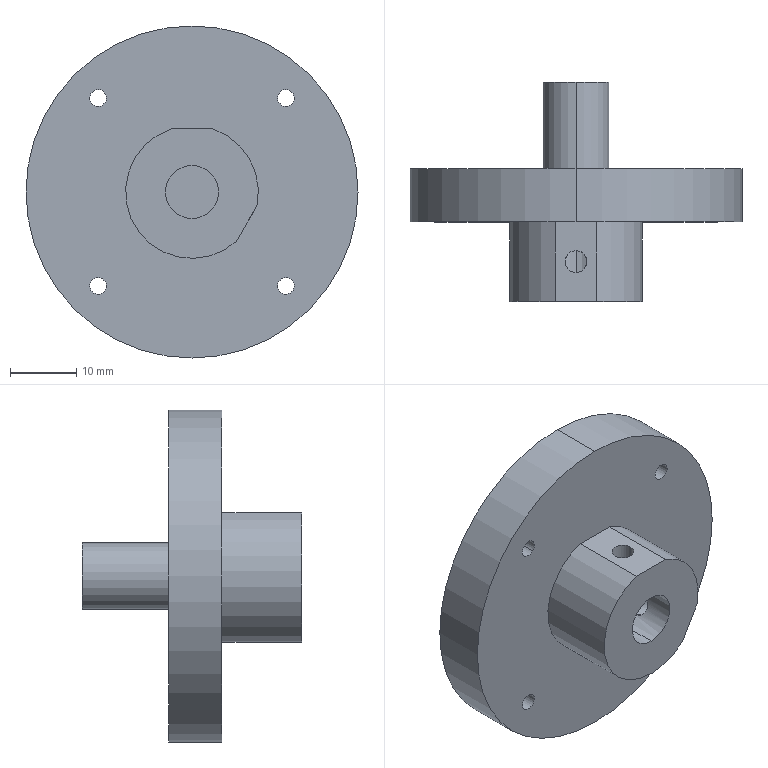Part | NX | features BREP 1 | 1 solid | 31 faces | box 50 x 33 x 50 mm | volume 19638 mm3 | cylinder 24 | plane 7 | commonest cylinder face diameters 2.5 x12 3.3 x4 8 x2 10 x2 20 x2 50 x2
STEP:
#1=CARTESIAN_POINT('',(-14.122,12.,15.412));
#2=VERTEX_POINT('',#1);
#3=CARTESIAN_POINT('',(-13.258,12.,13.258));
#4=VERTEX_POINT('',#3);
#5=CARTESIAN_POINT('',(-14.122,12.,14.162));
#6=DIRECTION('',(0.,1.,0.));
#7=DIRECTION('',(0.,0.,1.));
#8=AXIS2_PLACEMENT_3D('',#5,#6,#7);
#9=CIRCLE('',#8,1.25);
#10=EDGE_CURVE('',#2,#4,#9,.T.);
#11=ORIENTED_EDGE('',*,*,#10,.F.);
#12=CARTESIAN_POINT('',(-14.122,20.,15.412));
#13=VERTEX_POINT('',#12);
#14=CARTESIAN_POINT('',(-14.122,20.,15.412));
#15=DIRECTION('',(0.,1.,0.));
#16=VECTOR('',#15,1000.);
#17=LINE('',#14,#16);
#18=EDGE_CURVE('',#2,#13,#17,.T.);
#19=ORIENTED_EDGE('',*,*,#18,.T.);
#20=CARTESIAN_POINT('',(-13.258,20.,13.258));
#21=VERTEX_POINT('',#20);
#22=CARTESIAN_POINT('',(-14.122,20.,14.162));
#23=DIRECTION('',(0.,1.,0.));
#24=DIRECTION('',(0.,0.,1.));
#25=AXIS2_PLACEMENT_3D('',#22,#23,#24);
#26=CIRCLE('',#25,1.25);
#27=EDGE_CURVE('',#13,#21,#26,.T.);
#28=ORIENTED_EDGE('',*,*,#27,.T.);
#29=CARTESIAN_POINT('',(-13.258,10.,13.258));
#30=DIRECTION('',(0.,1.,0.));
#31=VECTOR('',#30,1000.);
#32=LINE('',#29,#31);
#33=EDGE_CURVE('',#4,#21,#32,.T.);
#34=ORIENTED_EDGE('',*,*,#33,.F.);
#35=EDGE_LOOP('',(#11,#19,#28,#34));
#36=FACE_BOUND('',#35,.T.);
#37=CARTESIAN_POINT('',(-14.122,20.,14.162));
#38=DIRECTION('',(0.,1.,0.));
#39=DIRECTION('',(0.,0.,-1.));
#40=AXIS2_PLACEMENT_3D('',#37,#38,#39);
#41=CYLINDRICAL_SURFACE('',#40,1.25);
#42=ADVANCED_FACE('',(#36),#41,.F.);
#43=CARTESIAN_POINT('',(-14.162,12.,-12.872));
#44=VERTEX_POINT('',#43);
#45=CARTESIAN_POINT('',(-13.258,12.,-13.258));
#46=VERTEX_POINT('',#45);
#47=CARTESIAN_POINT('',(-14.162,12.,-14.122));
#48=DIRECTION('',(0.,1.,0.));
#49=DIRECTION('',(0.,0.,1.));
#50=AXIS2_PLACEMENT_3D('',#47,#48,#49);
#51=CIRCLE('',#50,1.25);
#52=EDGE_CURVE('',#44,#46,#51,.T.);
#53=ORIENTED_EDGE('',*,*,#52,.F.);
#54=CARTESIAN_POINT('',(-14.162,20.,-12.872));
#55=VERTEX_POINT('',#54);
#56=CARTESIAN_POINT('',(-14.162,20.,-12.872));
#57=DIRECTION('',(0.,1.,0.));
#58=VECTOR('',#57,1000.);
#59=LINE('',#56,#58);
#60=EDGE_CURVE('',#44,#55,#59,.T.);
#61=ORIENTED_EDGE('',*,*,#60,.T.);
#62=CARTESIAN_POINT('',(-13.258,20.,-13.258));
#63=VERTEX_POINT('',#62);
#64=CARTESIAN_POINT('',(-14.162,20.,-14.122));
#65=DIRECTION('',(0.,1.,0.));
#66=DIRECTION('',(0.,0.,1.));
#67=AXIS2_PLACEMENT_3D('',#64,#65,#66);
#68=CIRCLE('',#67,1.25);
#69=EDGE_CURVE('',#55,#63,#68,.T.);
#70=ORIENTED_EDGE('',*,*,#69,.T.);
#71=CARTESIAN_POINT('',(-13.258,10.,-13.258));
#72=DIRECTION('',(0.,-1.,0.));
#73=VECTOR('',#72,1000.);
#74=LINE('',#71,#73);
#75=EDGE_CURVE('',#63,#46,#74,.T.);
#76=ORIENTED_EDGE('',*,*,#75,.T.);
#77=EDGE_LOOP('',(#53,#61,#70,#76));
#78=FACE_BOUND('',#77,.T.);
#79=CARTESIAN_POINT('',(-14.162,20.,-14.122));
#80=DIRECTION('',(0.,1.,0.));
#81=DIRECTION('',(0.,0.,-1.));
#82=AXIS2_PLACEMENT_3D('',#79,#80,#81);
#83=CYLINDRICAL_SURFACE('',#82,1.25);
#84=ADVANCED_FACE('',(#78),#83,.F.);
#85=CARTESIAN_POINT('',(14.162,12.,-12.872));
#86=VERTEX_POINT('',#85);
#87=CARTESIAN_POINT('',(15.026,12.,-15.026));
#88=VERTEX_POINT('',#87);
#89=CARTESIAN_POINT('',(14.162,12.,-14.122));
#90=DIRECTION('',(0.,1.,0.));
#91=DIRECTION('',(0.,0.,1.));
#92=AXIS2_PLACEMENT_3D('',#89,#90,#91);
#93=CIRCLE('',#92,1.25);
#94=EDGE_CURVE('',#86,#88,#93,.T.);
#95=ORIENTED_EDGE('',*,*,#94,.F.);
#96=CARTESIAN_POINT('',(14.162,20.,-12.872));
#97=VERTEX_POINT('',#96);
#98=CARTESIAN_POINT('',(14.162,20.,-12.872));
#99=DIRECTION('',(0.,1.,0.));
#100=VECTOR('',#99,1000.);
#101=LINE('',#98,#100);
#102=EDGE_CURVE('',#86,#97,#101,.T.);
#103=ORIENTED_EDGE('',*,*,#102,.T.);
#104=CARTESIAN_POINT('',(15.026,20.,-15.026));
#105=VERTEX_POINT('',#104);
#106=CARTESIAN_POINT('',(14.162,20.,-14.122));
#107=DIRECTION('',(0.,1.,0.));
#108=DIRECTION('',(0.,0.,1.));
#109=AXIS2_PLACEMENT_3D('',#106,#107,#108);
#110=CIRCLE('',#109,1.25);
#111=EDGE_CURVE('',#97,#105,#110,.T.);
#112=ORIENTED_EDGE('',*,*,#111,.T.);
#113=CARTESIAN_POINT('',(15.026,10.,-15.026));
#114=DIRECTION('',(0.,1.,0.));
#115=VECTOR('',#114,1000.);
#116=LINE('',#113,#115);
#117=EDGE_CURVE('',#88,#105,#116,.T.);
#118=ORIENTED_EDGE('',*,*,#117,.F.);
#119=EDGE_LOOP('',(#95,#103,#112,#118));
#120=FACE_BOUND('',#119,.T.);
#121=CARTESIAN_POINT('',(14.162,20.,-14.122));
#122=DIRECTION('',(0.,1.,0.));
#123=DIRECTION('',(0.,0.,-1.));
#124=AXIS2_PLACEMENT_3D('',#121,#122,#123);
#125=CYLINDRICAL_SURFACE('',#124,1.25);
#126=ADVANCED_FACE('',(#120),#125,.F.);
#127=CARTESIAN_POINT('',(14.122,12.,15.412));
#128=VERTEX_POINT('',#127);
#129=CARTESIAN_POINT('',(15.026,12.,15.026));
#130=VERTEX_POINT('',#129);
#131=CARTESIAN_POINT('',(14.122,12.,14.162));
#132=DIRECTION('',(0.,1.,0.));
#133=DIRECTION('',(0.,0.,1.));
#134=AXIS2_PLACEMENT_3D('',#131,#132,#133);
#135=CIRCLE('',#134,1.25);
#136=EDGE_CURVE('',#128,#130,#135,.T.);
#137=ORIENTED_EDGE('',*,*,#136,.F.);
#138=CARTESIAN_POINT('',(14.122,20.,15.412));
#139=VERTEX_POINT('',#138);
#140=CARTESIAN_POINT('',(14.122,20.,15.412));
#141=DIRECTION('',(0.,1.,0.));
#142=VECTOR('',#141,1000.);
#143=LINE('',#140,#142);
#144=EDGE_CURVE('',#128,#139,#143,.T.);
#145=ORIENTED_EDGE('',*,*,#144,.T.);
#146=CARTESIAN_POINT('',(15.026,20.,15.026));
#147=VERTEX_POINT('',#146);
#148=CARTESIAN_POINT('',(14.122,20.,14.162));
#149=DIRECTION('',(0.,1.,0.));
#150=DIRECTION('',(0.,0.,1.));
#151=AXIS2_PLACEMENT_3D('',#148,#149,#150);
#152=CIRCLE('',#151,1.25);
#153=EDGE_CURVE('',#139,#147,#152,.T.);
#154=ORIENTED_EDGE('',*,*,#153,.T.);
#155=CARTESIAN_POINT('',(15.026,10.,15.026));
#156=DIRECTION('',(0.,1.,0.));
#157=VECTOR('',#156,1000.);
#158=LINE('',#155,#157);
#159=EDGE_CURVE('',#130,#147,#158,.T.);
#160=ORIENTED_EDGE('',*,*,#159,.F.);
#161=EDGE_LOOP('',(#137,#145,#154,#160));
#162=FACE_BOUND('',#161,.T.);
#163=CARTESIAN_POINT('',(14.122,20.,14.162));
#164=DIRECTION('',(0.,1.,0.));
#165=DIRECTION('',(0.,0.,-1.));
#166=AXIS2_PLACEMENT_3D('',#163,#164,#165);
#167=CYLINDRICAL_SURFACE('',#166,1.25);
#168=ADVANCED_FACE('',(#162),#167,.F.);
#169=CARTESIAN_POINT('',(0.,33.,5.));
#170=VERTEX_POINT('',#169);
#171=CARTESIAN_POINT('',(0.,33.,-5.));
#172=VERTEX_POINT('',#171);
#173=CARTESIAN_POINT('',(0.,33.,0.));
#174=DIRECTION('',(0.,1.,0.));
#175=DIRECTION('',(0.,0.,1.));
#176=AXIS2_PLACEMENT_3D('',#173,#174,#175);
#177=CIRCLE('',#176,5.);
#178=EDGE_CURVE('',#170,#172,#177,.T.);
#179=ORIENTED_EDGE('',*,*,#178,.F.);
#180=CARTESIAN_POINT('',(0.,20.,5.));
#181=VERTEX_POINT('',#180);
#182=CARTESIAN_POINT('',(0.,33.,5.));
#183=DIRECTION('',(0.,-1.,0.));
#184=VECTOR('',#183,1000.);
#185=LINE('',#182,#184);
#186=EDGE_CURVE('',#181,#170,#185,.F.);
#187=ORIENTED_EDGE('',*,*,#186,.F.);
#188=CARTESIAN_POINT('',(0.,20.,-5.));
#189=VERTEX_POINT('',#188);
#190=CARTESIAN_POINT('',(0.,20.,0.));
#191=DIRECTION('',(0.,1.,0.));
#192=DIRECTION('',(0.,0.,-1.));
#193=AXIS2_PLACEMENT_3D('',#190,#191,#192);
#194=CIRCLE('',#193,5.);
#195=EDGE_CURVE('',#181,#189,#194,.T.);
#196=ORIENTED_EDGE('',*,*,#195,.T.);
#197=CARTESIAN_POINT('',(0.,33.,-5.));
#198=DIRECTION('',(0.,-1.,0.));
#199=VECTOR('',#198,1000.);
#200=LINE('',#197,#199);
#201=EDGE_CURVE('',#189,#172,#200,.F.);
#202=ORIENTED_EDGE('',*,*,#201,.T.);
#203=EDGE_LOOP('',(#179,#187,#196,#202));
#204=FACE_BOUND('',#203,.T.);
#205=CARTESIAN_POINT('',(0.,33.,0.));
#206=DIRECTION('',(0.,-1.,0.));
#207=DIRECTION('',(0.,0.,1.));
#208=AXIS2_PLACEMENT_3D('',#205,#206,#207);
#209=CYLINDRICAL_SURFACE('',#208,5.);
#210=ADVANCED_FACE('',(#204),#209,.T.);
#211=CARTESIAN_POINT('',(3.981,6.,-0.393));
#212=VERTEX_POINT('',#211);
#213=CARTESIAN_POINT('',(2.331,6.,-3.251));
#214=VERTEX_POINT('',#213);
#215=CARTESIAN_POINT('',(3.981,6.,-0.393));
#216=CARTESIAN_POINT('',(3.981,5.559,-0.393));
#217=CARTESIAN_POINT('',(3.963,4.713,-0.7955));
#218=CARTESIAN_POINT('',(3.539,4.169,-2.039));
#219=CARTESIAN_POINT('',(2.67,4.712,-3.036));
#220=CARTESIAN_POINT('',(2.331,5.559,-3.251));
#221=CARTESIAN_POINT('',(2.331,6.,-3.251));
#222=B_SPLINE_CURVE_WITH_KNOTS('',3,(#215,#216,#217,#218,#219,#220,#221),.UNSPECIFIED.,.F.,.F.,(4,1,1,1,4),(0.,0.001304,0.002607,0.003911,0.005215),.UNSPECIFIED.);
#223=EDGE_CURVE('',#212,#214,#222,.T.);
#224=ORIENTED_EDGE('',*,*,#223,.F.);
#225=CARTESIAN_POINT('',(9.052,6.,-3.321));
#226=VERTEX_POINT('',#225);
#227=CARTESIAN_POINT('',(9.485,6.,-3.571));
#228=DIRECTION('',(0.866,0.,-0.5));
#229=VECTOR('',#228,1000.);
#230=LINE('',#227,#229);
#231=EDGE_CURVE('',#226,#212,#230,.F.);
#232=ORIENTED_EDGE('',*,*,#231,.F.);
#233=CARTESIAN_POINT('',(7.402,6.,-6.179));
#234=VERTEX_POINT('',#233);
#235=CARTESIAN_POINT('',(8.227,6.,-4.75));
#236=DIRECTION('',(0.866,0.,-0.5));
#237=DIRECTION('',(0.5,0.,0.866));
#238=AXIS2_PLACEMENT_3D('',#235,#236,#237);
#239=CIRCLE('',#238,1.65);
#240=EDGE_CURVE('',#226,#234,#239,.T.);
#241=ORIENTED_EDGE('',*,*,#240,.T.);
#242=CARTESIAN_POINT('',(7.835,6.,-6.429));
#243=DIRECTION('',(0.866,0.,-0.5));
#244=VECTOR('',#243,1000.);
#245=LINE('',#242,#244);
#246=EDGE_CURVE('',#234,#214,#245,.F.);
#247=ORIENTED_EDGE('',*,*,#246,.T.);
#248=EDGE_LOOP('',(#224,#232,#241,#247));
#249=FACE_BOUND('',#248,.T.);
#250=CARTESIAN_POINT('',(8.66,6.,-5.));
#251=DIRECTION('',(0.866,0.,-0.5));
#252=DIRECTION('',(0.5,0.,0.866));
#253=AXIS2_PLACEMENT_3D('',#250,#251,#252);
#254=CYLINDRICAL_SURFACE('',#253,1.65);
#255=ADVANCED_FACE('',(#249),#254,.F.);
#256=CARTESIAN_POINT('',(-1.65,6.,3.644));
#257=VERTEX_POINT('',#256);
#258=CARTESIAN_POINT('',(0.,4.35,4.));
#259=VERTEX_POINT('',#258);
#260=CARTESIAN_POINT('',(-1.65,6.,3.644));
#261=CARTESIAN_POINT('',(-1.65,5.118,3.644));
#262=CARTESIAN_POINT('',(-0.8824,4.35,4.));
#263=CARTESIAN_POINT('',(0.,4.35,4.));
#264=B_SPLINE_CURVE_WITH_KNOTS('',3,(#260,#261,#262,#263),.UNSPECIFIED.,.F.,.F.,(4,4),(0.,0.002607),.UNSPECIFIED.);
#265=EDGE_CURVE('',#257,#259,#264,.T.);
#266=ORIENTED_EDGE('',*,*,#265,.F.);
#267=CARTESIAN_POINT('',(-1.65,6.,9.5));
#268=VERTEX_POINT('',#267);
#269=CARTESIAN_POINT('',(-1.65,6.,10.));
#270=DIRECTION('',(0.,0.,1.));
#271=VECTOR('',#270,1000.);
#272=LINE('',#269,#271);
#273=EDGE_CURVE('',#257,#268,#272,.T.);
#274=ORIENTED_EDGE('',*,*,#273,.T.);
#275=CARTESIAN_POINT('',(1.65,6.,9.5));
#276=VERTEX_POINT('',#275);
#277=CARTESIAN_POINT('',(0.,6.,9.5));
#278=DIRECTION('',(0.,0.,1.));
#279=DIRECTION('',(-1.,0.,0.));
#280=AXIS2_PLACEMENT_3D('',#277,#278,#279);
#281=CIRCLE('',#280,1.65);
#282=EDGE_CURVE('',#268,#276,#281,.T.);
#283=ORIENTED_EDGE('',*,*,#282,.T.);
#284=CARTESIAN_POINT('',(1.65,6.,3.644));
#285=VERTEX_POINT('',#284);
#286=CARTESIAN_POINT('',(1.65,6.,10.));
#287=DIRECTION('',(0.,0.,1.));
#288=VECTOR('',#287,1000.);
#289=LINE('',#286,#288);
#290=EDGE_CURVE('',#285,#276,#289,.T.);
#291=ORIENTED_EDGE('',*,*,#290,.F.);
#292=CARTESIAN_POINT('',(0.,4.35,4.));
#293=CARTESIAN_POINT('',(0.8823,4.35,4.));
#294=CARTESIAN_POINT('',(1.65,5.118,3.644));
#295=CARTESIAN_POINT('',(1.65,6.,3.644));
#296=B_SPLINE_CURVE_WITH_KNOTS('',3,(#292,#293,#294,#295),.UNSPECIFIED.,.F.,.F.,(4,4),(0.,0.002607),.UNSPECIFIED.);
#297=EDGE_CURVE('',#259,#285,#296,.T.);
#298=ORIENTED_EDGE('',*,*,#297,.F.);
#299=EDGE_LOOP('',(#266,#274,#283,#291,#298));
#300=FACE_BOUND('',#299,.T.);
#301=CARTESIAN_POINT('',(0.,6.,10.));
#302=DIRECTION('',(0.,0.,1.));
#303=DIRECTION('',(-1.,0.,0.));
#304=AXIS2_PLACEMENT_3D('',#301,#302,#303);
#305=CYLINDRICAL_SURFACE('',#304,1.65);
#306=ADVANCED_FACE('',(#300),#305,.F.);
#307=CARTESIAN_POINT('',(0.,11.,4.));
#308=VERTEX_POINT('',#307);
#309=CARTESIAN_POINT('',(0.,11.,-4.));
#310=VERTEX_POINT('',#309);
#311=CARTESIAN_POINT('',(0.,11.,0.));
#312=DIRECTION('',(0.,-1.,0.));
#313=DIRECTION('',(0.,0.,-1.));
#314=AXIS2_PLACEMENT_3D('',#311,#312,#313);
#315=CIRCLE('',#314,4.);
#316=EDGE_CURVE('',#308,#310,#315,.T.);
#317=ORIENTED_EDGE('',*,*,#316,.F.);
#318=CARTESIAN_POINT('',(0.,7.65,4.));
#319=VERTEX_POINT('',#318);
#320=CARTESIAN_POINT('',(0.,11.,4.));
#321=DIRECTION('',(0.,-1.,0.));
#322=VECTOR('',#321,1000.);
#323=LINE('',#320,#322);
#324=EDGE_CURVE('',#319,#308,#323,.F.);
#325=ORIENTED_EDGE('',*,*,#324,.F.);
#326=CARTESIAN_POINT('',(0.,7.65,4.));
#327=CARTESIAN_POINT('',(-0.8823,7.65,4.));
#328=CARTESIAN_POINT('',(-1.65,6.882,3.644));
#329=CARTESIAN_POINT('',(-1.65,6.,3.644));
#330=B_SPLINE_CURVE_WITH_KNOTS('',3,(#326,#327,#328,#329),.UNSPECIFIED.,.F.,.F.,(4,4),(0.,0.002607),.UNSPECIFIED.);
#331=EDGE_CURVE('',#319,#257,#330,.T.);
#332=ORIENTED_EDGE('',*,*,#331,.T.);
#333=ORIENTED_EDGE('',*,*,#265,.T.);
#334=CARTESIAN_POINT('',(0.,0.,4.));
#335=VERTEX_POINT('',#334);
#336=CARTESIAN_POINT('',(0.,11.,4.));
#337=DIRECTION('',(0.,-1.,0.));
#338=VECTOR('',#337,1000.);
#339=LINE('',#336,#338);
#340=EDGE_CURVE('',#259,#335,#339,.T.);
#341=ORIENTED_EDGE('',*,*,#340,.T.);
#342=CARTESIAN_POINT('',(0.,0.,-4.));
#343=VERTEX_POINT('',#342);
#344=CARTESIAN_POINT('',(0.,0.,0.));
#345=DIRECTION('',(0.,-1.,0.));
#346=DIRECTION('',(0.,0.,-1.));
#347=AXIS2_PLACEMENT_3D('',#344,#345,#346);
#348=CIRCLE('',#347,4.);
#349=EDGE_CURVE('',#335,#343,#348,.T.);
#350=ORIENTED_EDGE('',*,*,#349,.T.);
#351=CARTESIAN_POINT('',(0.,11.,-4.));
#352=DIRECTION('',(0.,-1.,0.));
#353=VECTOR('',#352,1000.);
#354=LINE('',#351,#353);
#355=EDGE_CURVE('',#343,#310,#354,.F.);
#356=ORIENTED_EDGE('',*,*,#355,.T.);
#357=EDGE_LOOP('',(#317,#325,#332,#333,#341,#350,#356));
#358=FACE_BOUND('',#357,.T.);
#359=CARTESIAN_POINT('',(0.,11.,0.));
#360=DIRECTION('',(0.,-1.,0.));
#361=DIRECTION('',(0.,0.,1.));
#362=AXIS2_PLACEMENT_3D('',#359,#360,#361);
#363=CYLINDRICAL_SURFACE('',#362,4.);
#364=ADVANCED_FACE('',(#358),#363,.F.);
#365=CARTESIAN_POINT('',(0.,12.,25.));
#366=VERTEX_POINT('',#365);
#367=CARTESIAN_POINT('',(0.,12.,-25.));
#368=VERTEX_POINT('',#367);
#369=CARTESIAN_POINT('',(0.,12.,0.));
#370=DIRECTION('',(0.,1.,0.));
#371=DIRECTION('',(0.,0.,1.));
#372=AXIS2_PLACEMENT_3D('',#369,#370,#371);
#373=CIRCLE('',#372,25.);
#374=EDGE_CURVE('',#366,#368,#373,.T.);
#375=ORIENTED_EDGE('',*,*,#374,.T.);
#376=CARTESIAN_POINT('',(0.,20.,-25.));
#377=VERTEX_POINT('',#376);
#378=CARTESIAN_POINT('',(0.,81.449,-25.));
#379=DIRECTION('',(0.,1.,0.));
#380=VECTOR('',#379,1000.);
#381=LINE('',#378,#380);
#382=EDGE_CURVE('',#368,#377,#381,.T.);
#383=ORIENTED_EDGE('',*,*,#382,.T.);
#384=CARTESIAN_POINT('',(0.,20.,25.));
#385=VERTEX_POINT('',#384);
#386=CARTESIAN_POINT('',(0.,20.,0.));
#387=DIRECTION('',(0.,1.,0.));
#388=DIRECTION('',(0.,0.,1.));
#389=AXIS2_PLACEMENT_3D('',#386,#387,#388);
#390=CIRCLE('',#389,25.);
#391=EDGE_CURVE('',#385,#377,#390,.T.);
#392=ORIENTED_EDGE('',*,*,#391,.F.);
#393=CARTESIAN_POINT('',(0.,81.449,25.));
#394=DIRECTION('',(0.,1.,0.));
#395=VECTOR('',#394,1000.);
#396=LINE('',#393,#395);
#397=EDGE_CURVE('',#366,#385,#396,.T.);
#398=ORIENTED_EDGE('',*,*,#397,.F.);
#399=EDGE_LOOP('',(#375,#383,#392,#398));
#400=FACE_BOUND('',#399,.T.);
#401=CARTESIAN_POINT('',(0.,81.449,0.));
#402=DIRECTION('',(0.,1.,0.));
#403=DIRECTION('',(0.,0.,-1.));
#404=AXIS2_PLACEMENT_3D('',#401,#402,#403);
#405=CYLINDRICAL_SURFACE('',#404,25.);
#406=ADVANCED_FACE('',(#400),#405,.T.);
#407=CARTESIAN_POINT('',(-15.026,20.,-15.026));
#408=VERTEX_POINT('',#407);
#409=CARTESIAN_POINT('',(-14.122,20.,-14.162));
#410=DIRECTION('',(0.,1.,0.));
#411=DIRECTION('',(0.,0.,1.));
#412=AXIS2_PLACEMENT_3D('',#409,#410,#411);
#413=CIRCLE('',#412,1.25);
#414=EDGE_CURVE('',#63,#408,#413,.T.);
#415=ORIENTED_EDGE('',*,*,#414,.F.);
#416=ORIENTED_EDGE('',*,*,#69,.F.);
#417=CARTESIAN_POINT('',(-14.162,20.,-14.122));
#418=DIRECTION('',(0.,1.,0.));
#419=DIRECTION('',(0.,0.,1.));
#420=AXIS2_PLACEMENT_3D('',#417,#418,#419);
#421=CIRCLE('',#420,1.25);
#422=EDGE_CURVE('',#408,#55,#421,.T.);
#423=ORIENTED_EDGE('',*,*,#422,.F.);
#424=EDGE_LOOP('',(#415,#416,#423));
#425=FACE_BOUND('',#424,.T.);
#426=CARTESIAN_POINT('',(13.258,20.,-13.258));
#427=VERTEX_POINT('',#426);
#428=CARTESIAN_POINT('',(14.122,20.,-14.162));
#429=DIRECTION('',(0.,1.,0.));
#430=DIRECTION('',(0.,0.,1.));
#431=AXIS2_PLACEMENT_3D('',#428,#429,#430);
#432=CIRCLE('',#431,1.25);
#433=EDGE_CURVE('',#105,#427,#432,.T.);
#434=ORIENTED_EDGE('',*,*,#433,.F.);
#435=ORIENTED_EDGE('',*,*,#111,.F.);
#436=CARTESIAN_POINT('',(14.162,20.,-14.122));
#437=DIRECTION('',(0.,1.,0.));
#438=DIRECTION('',(0.,0.,1.));
#439=AXIS2_PLACEMENT_3D('',#436,#437,#438);
#440=CIRCLE('',#439,1.25);
#441=EDGE_CURVE('',#427,#97,#440,.T.);
#442=ORIENTED_EDGE('',*,*,#441,.F.);
#443=EDGE_LOOP('',(#434,#435,#442));
#444=FACE_BOUND('',#443,.T.);
#445=CARTESIAN_POINT('',(13.258,20.,13.258));
#446=VERTEX_POINT('',#445);
#447=CARTESIAN_POINT('',(14.162,20.,14.122));
#448=DIRECTION('',(0.,1.,0.));
#449=DIRECTION('',(0.,0.,1.));
#450=AXIS2_PLACEMENT_3D('',#447,#448,#449);
#451=CIRCLE('',#450,1.25);
#452=EDGE_CURVE('',#147,#446,#451,.T.);
#453=ORIENTED_EDGE('',*,*,#452,.F.);
#454=ORIENTED_EDGE('',*,*,#153,.F.);
#455=CARTESIAN_POINT('',(14.122,20.,14.162));
#456=DIRECTION('',(0.,1.,0.));
#457=DIRECTION('',(0.,0.,1.));
#458=AXIS2_PLACEMENT_3D('',#455,#456,#457);
#459=CIRCLE('',#458,1.25);
#460=EDGE_CURVE('',#446,#139,#459,.T.);
#461=ORIENTED_EDGE('',*,*,#460,.F.);
#462=EDGE_LOOP('',(#453,#454,#461));
#463=FACE_BOUND('',#462,.T.);
#464=CARTESIAN_POINT('',(0.,20.,0.));
#465=DIRECTION('',(0.,1.,0.));
#466=DIRECTION('',(0.,0.,-1.));
#467=AXIS2_PLACEMENT_3D('',#464,#465,#466);
#468=CIRCLE('',#467,5.);
#469=EDGE_CURVE('',#189,#181,#468,.T.);
#470=ORIENTED_EDGE('',*,*,#469,.F.);
#471=ORIENTED_EDGE('',*,*,#195,.F.);
#472=EDGE_LOOP('',(#470,#471));
#473=FACE_BOUND('',#472,.T.);
#474=ORIENTED_EDGE('',*,*,#391,.T.);
#475=CARTESIAN_POINT('',(0.,20.,0.));
#476=DIRECTION('',(0.,1.,0.));
#477=DIRECTION('',(0.,0.,1.));
#478=AXIS2_PLACEMENT_3D('',#475,#476,#477);
#479=CIRCLE('',#478,25.);
#480=EDGE_CURVE('',#377,#385,#479,.T.);
#481=ORIENTED_EDGE('',*,*,#480,.T.);
#482=EDGE_LOOP('',(#474,#481));
#483=FACE_BOUND('',#482,.T.);
#484=CARTESIAN_POINT('',(-15.026,20.,15.026));
#485=VERTEX_POINT('',#484);
#486=CARTESIAN_POINT('',(-14.122,20.,14.162));
#487=DIRECTION('',(0.,1.,0.));
#488=DIRECTION('',(0.,0.,1.));
#489=AXIS2_PLACEMENT_3D('',#486,#487,#488);
#490=CIRCLE('',#489,1.25);
#491=EDGE_CURVE('',#485,#13,#490,.T.);
#492=ORIENTED_EDGE('',*,*,#491,.F.);
#493=CARTESIAN_POINT('',(-14.162,20.,14.122));
#494=DIRECTION('',(0.,1.,0.));
#495=DIRECTION('',(0.,0.,1.));
#496=AXIS2_PLACEMENT_3D('',#493,#494,#495);
#497=CIRCLE('',#496,1.25);
#498=EDGE_CURVE('',#21,#485,#497,.T.);
#499=ORIENTED_EDGE('',*,*,#498,.F.);
#500=ORIENTED_EDGE('',*,*,#27,.F.);
#501=EDGE_LOOP('',(#492,#499,#500));
#502=FACE_BOUND('',#501,.T.);
#503=CARTESIAN_POINT('',(0.,20.,0.));
#504=DIRECTION('',(0.,-1.,0.));
#505=DIRECTION('',(0.,0.,1.));
#506=AXIS2_PLACEMENT_3D('',#503,#504,#505);
#507=PLANE('',#506);
#508=ADVANCED_FACE('',(#425,#444,#463,#473,#483,#502),#507,.F.);
#509=CARTESIAN_POINT('',(3.122,0.,9.5));
#510=VERTEX_POINT('',#509);
#511=CARTESIAN_POINT('',(9.788,0.,-2.046));
#512=VERTEX_POINT('',#511);
#513=CARTESIAN_POINT('',(0.,0.,0.));
#514=DIRECTION('',(0.,1.,0.));
#515=DIRECTION('',(0.,0.,1.));
#516=AXIS2_PLACEMENT_3D('',#513,#514,#515);
#517=CIRCLE('',#516,10.);
#518=EDGE_CURVE('',#510,#512,#517,.T.);
#519=ORIENTED_EDGE('',*,*,#518,.T.);
#520=CARTESIAN_POINT('',(9.788,12.,-2.046));
#521=VERTEX_POINT('',#520);
#522=CARTESIAN_POINT('',(9.788,18.245,-2.046));
#523=DIRECTION('',(0.,-1.,0.));
#524=VECTOR('',#523,1000.);
#525=LINE('',#522,#524);
#526=EDGE_CURVE('',#521,#512,#525,.T.);
#527=ORIENTED_EDGE('',*,*,#526,.F.);
#528=CARTESIAN_POINT('',(3.122,12.,9.5));
#529=VERTEX_POINT('',#528);
#530=CARTESIAN_POINT('',(0.,12.,0.));
#531=DIRECTION('',(0.,1.,0.));
#532=DIRECTION('',(0.,0.,1.));
#533=AXIS2_PLACEMENT_3D('',#530,#531,#532);
#534=CIRCLE('',#533,10.);
#535=EDGE_CURVE('',#529,#521,#534,.T.);
#536=ORIENTED_EDGE('',*,*,#535,.F.);
#537=CARTESIAN_POINT('',(3.122,18.265,9.5));
#538=DIRECTION('',(0.,-1.,0.));
#539=VECTOR('',#538,1000.);
#540=LINE('',#537,#539);
#541=EDGE_CURVE('',#529,#510,#540,.T.);
#542=ORIENTED_EDGE('',*,*,#541,.T.);
#543=EDGE_LOOP('',(#519,#527,#536,#542));
#544=FACE_BOUND('',#543,.T.);
#545=CARTESIAN_POINT('',(0.,81.449,0.));
#546=DIRECTION('',(0.,1.,0.));
#547=DIRECTION('',(0.,0.,-1.));
#548=AXIS2_PLACEMENT_3D('',#545,#546,#547);
#549=CYLINDRICAL_SURFACE('',#548,10.);
#550=ADVANCED_FACE('',(#544),#549,.T.);
#551=ORIENTED_EDGE('',*,*,#382,.F.);
#552=CARTESIAN_POINT('',(0.,12.,0.));
#553=DIRECTION('',(0.,1.,0.));
#554=DIRECTION('',(0.,0.,1.));
#555=AXIS2_PLACEMENT_3D('',#552,#553,#554);
#556=CIRCLE('',#555,25.);
#557=EDGE_CURVE('',#368,#366,#556,.T.);
#558=ORIENTED_EDGE('',*,*,#557,.T.);
#559=ORIENTED_EDGE('',*,*,#397,.T.);
#560=ORIENTED_EDGE('',*,*,#480,.F.);
#561=EDGE_LOOP('',(#551,#558,#559,#560));
#562=FACE_BOUND('',#561,.T.);
#563=CARTESIAN_POINT('',(0.,81.449,0.));
#564=DIRECTION('',(0.,1.,0.));
#565=DIRECTION('',(0.,0.,-1.));
#566=AXIS2_PLACEMENT_3D('',#563,#564,#565);
#567=CYLINDRICAL_SURFACE('',#566,25.);
#568=ADVANCED_FACE('',(#562),#567,.T.);
#569=CARTESIAN_POINT('',(-15.026,12.,-15.026));
#570=VERTEX_POINT('',#569);
#571=CARTESIAN_POINT('',(-14.162,12.,-14.122));
#572=DIRECTION('',(0.,1.,0.));
#573=DIRECTION('',(0.,0.,1.));
#574=AXIS2_PLACEMENT_3D('',#571,#572,#573);
#575=CIRCLE('',#574,1.25);
#576=EDGE_CURVE('',#570,#44,#575,.T.);
#577=ORIENTED_EDGE('',*,*,#576,.T.);
#578=ORIENTED_EDGE('',*,*,#52,.T.);
#579=CARTESIAN_POINT('',(-14.122,12.,-14.162));
#580=DIRECTION('',(0.,1.,0.));
#581=DIRECTION('',(0.,0.,1.));
#582=AXIS2_PLACEMENT_3D('',#579,#580,#581);
#583=CIRCLE('',#582,1.25);
#584=EDGE_CURVE('',#46,#570,#583,.T.);
#585=ORIENTED_EDGE('',*,*,#584,.T.);
#586=EDGE_LOOP('',(#577,#578,#585));
#587=FACE_BOUND('',#586,.T.);
#588=CARTESIAN_POINT('',(13.258,12.,-13.258));
#589=VERTEX_POINT('',#588);
#590=CARTESIAN_POINT('',(14.122,12.,-14.162));
#591=DIRECTION('',(0.,1.,0.));
#592=DIRECTION('',(0.,0.,1.));
#593=AXIS2_PLACEMENT_3D('',#590,#591,#592);
#594=CIRCLE('',#593,1.25);
#595=EDGE_CURVE('',#88,#589,#594,.T.);
#596=ORIENTED_EDGE('',*,*,#595,.T.);
#597=CARTESIAN_POINT('',(14.162,12.,-14.122));
#598=DIRECTION('',(0.,1.,0.));
#599=DIRECTION('',(0.,0.,1.));
#600=AXIS2_PLACEMENT_3D('',#597,#598,#599);
#601=CIRCLE('',#600,1.25);
#602=EDGE_CURVE('',#589,#86,#601,.T.);
#603=ORIENTED_EDGE('',*,*,#602,.T.);
#604=ORIENTED_EDGE('',*,*,#94,.T.);
#605=EDGE_LOOP('',(#596,#603,#604));
#606=FACE_BOUND('',#605,.T.);
#607=CARTESIAN_POINT('',(13.258,12.,13.258));
#608=VERTEX_POINT('',#607);
#609=CARTESIAN_POINT('',(14.162,12.,14.122));
#610=DIRECTION('',(0.,1.,0.));
#611=DIRECTION('',(0.,0.,1.));
#612=AXIS2_PLACEMENT_3D('',#609,#610,#611);
#613=CIRCLE('',#612,1.25);
#614=EDGE_CURVE('',#130,#608,#613,.T.);
#615=ORIENTED_EDGE('',*,*,#614,.T.);
#616=CARTESIAN_POINT('',(14.122,12.,14.162));
#617=DIRECTION('',(0.,1.,0.));
#618=DIRECTION('',(0.,0.,1.));
#619=AXIS2_PLACEMENT_3D('',#616,#617,#618);
#620=CIRCLE('',#619,1.25);
#621=EDGE_CURVE('',#608,#128,#620,.T.);
#622=ORIENTED_EDGE('',*,*,#621,.T.);
#623=ORIENTED_EDGE('',*,*,#136,.T.);
#624=EDGE_LOOP('',(#615,#622,#623));
#625=FACE_BOUND('',#624,.T.);
#626=CARTESIAN_POINT('',(-15.026,12.,15.026));
#627=VERTEX_POINT('',#626);
#628=CARTESIAN_POINT('',(-14.162,12.,14.122));
#629=DIRECTION('',(0.,1.,0.));
#630=DIRECTION('',(0.,0.,1.));
#631=AXIS2_PLACEMENT_3D('',#628,#629,#630);
#632=CIRCLE('',#631,1.25);
#633=EDGE_CURVE('',#4,#627,#632,.T.);
#634=ORIENTED_EDGE('',*,*,#633,.T.);
#635=CARTESIAN_POINT('',(-14.122,12.,14.162));
#636=DIRECTION('',(0.,1.,0.));
#637=DIRECTION('',(0.,0.,1.));
#638=AXIS2_PLACEMENT_3D('',#635,#636,#637);
#639=CIRCLE('',#638,1.25);
#640=EDGE_CURVE('',#627,#2,#639,.T.);
#641=ORIENTED_EDGE('',*,*,#640,.T.);
#642=ORIENTED_EDGE('',*,*,#10,.T.);
#643=EDGE_LOOP('',(#634,#641,#642));
#644=FACE_BOUND('',#643,.T.);
#645=ORIENTED_EDGE('',*,*,#374,.F.);
#646=ORIENTED_EDGE('',*,*,#557,.F.);
#647=EDGE_LOOP('',(#645,#646));
#648=FACE_BOUND('',#647,.T.);
#649=ORIENTED_EDGE('',*,*,#535,.T.);
#650=CARTESIAN_POINT('',(6.666,12.,-7.454));
#651=VERTEX_POINT('',#650);
#652=CARTESIAN_POINT('',(9.788,12.,-2.046));
#653=DIRECTION('',(-0.5,0.,-0.866));
#654=VECTOR('',#653,1000.);
#655=LINE('',#652,#654);
#656=EDGE_CURVE('',#521,#651,#655,.T.);
#657=ORIENTED_EDGE('',*,*,#656,.T.);
#658=CARTESIAN_POINT('',(-3.122,12.,9.5));
#659=VERTEX_POINT('',#658);
#660=CARTESIAN_POINT('',(0.,12.,0.));
#661=DIRECTION('',(0.,1.,0.));
#662=DIRECTION('',(0.,0.,1.));
#663=AXIS2_PLACEMENT_3D('',#660,#661,#662);
#664=CIRCLE('',#663,10.);
#665=EDGE_CURVE('',#651,#659,#664,.T.);
#666=ORIENTED_EDGE('',*,*,#665,.T.);
#667=CARTESIAN_POINT('',(-3.122,12.,9.5));
#668=DIRECTION('',(1.,0.,0.));
#669=VECTOR('',#668,1000.);
#670=LINE('',#667,#669);
#671=EDGE_CURVE('',#659,#529,#670,.T.);
#672=ORIENTED_EDGE('',*,*,#671,.T.);
#673=EDGE_LOOP('',(#649,#657,#666,#672));
#674=FACE_BOUND('',#673,.T.);
#675=CARTESIAN_POINT('',(25.,12.,0.));
#676=DIRECTION('',(0.,1.,0.));
#677=DIRECTION('',(0.,0.,-1.));
#678=AXIS2_PLACEMENT_3D('',#675,#676,#677);
#679=PLANE('',#678);
#680=ADVANCED_FACE('',(#587,#606,#625,#644,#648,#674),#679,.F.);
#681=ORIENTED_EDGE('',*,*,#665,.F.);
#682=CARTESIAN_POINT('',(6.666,0.,-7.454));
#683=VERTEX_POINT('',#682);
#684=CARTESIAN_POINT('',(6.666,18.245,-7.454));
#685=DIRECTION('',(0.,-1.,0.));
#686=VECTOR('',#685,1000.);
#687=LINE('',#684,#686);
#688=EDGE_CURVE('',#651,#683,#687,.T.);
#689=ORIENTED_EDGE('',*,*,#688,.T.);
#690=CARTESIAN_POINT('',(-3.122,0.,9.5));
#691=VERTEX_POINT('',#690);
#692=CARTESIAN_POINT('',(0.,0.,0.));
#693=DIRECTION('',(0.,1.,0.));
#694=DIRECTION('',(0.,0.,1.));
#695=AXIS2_PLACEMENT_3D('',#692,#693,#694);
#696=CIRCLE('',#695,10.);
#697=EDGE_CURVE('',#683,#691,#696,.T.);
#698=ORIENTED_EDGE('',*,*,#697,.T.);
#699=CARTESIAN_POINT('',(-3.122,18.265,9.5));
#700=DIRECTION('',(0.,-1.,0.));
#701=VECTOR('',#700,1000.);
#702=LINE('',#699,#701);
#703=EDGE_CURVE('',#659,#691,#702,.T.);
#704=ORIENTED_EDGE('',*,*,#703,.F.);
#705=EDGE_LOOP('',(#681,#689,#698,#704));
#706=FACE_BOUND('',#705,.T.);
#707=CARTESIAN_POINT('',(0.,81.449,0.));
#708=DIRECTION('',(0.,1.,0.));
#709=DIRECTION('',(0.,0.,-1.));
#710=AXIS2_PLACEMENT_3D('',#707,#708,#709);
#711=CYLINDRICAL_SURFACE('',#710,10.);
#712=ADVANCED_FACE('',(#706),#711,.T.);
#713=CARTESIAN_POINT('',(0.,0.,0.));
#714=DIRECTION('',(0.,-1.,0.));
#715=DIRECTION('',(0.,0.,-1.));
#716=AXIS2_PLACEMENT_3D('',#713,#714,#715);
#717=CIRCLE('',#716,4.);
#718=EDGE_CURVE('',#343,#335,#717,.T.);
#719=ORIENTED_EDGE('',*,*,#718,.F.);
#720=ORIENTED_EDGE('',*,*,#349,.F.);
#721=EDGE_LOOP('',(#719,#720));
#722=FACE_BOUND('',#721,.T.);
#723=ORIENTED_EDGE('',*,*,#697,.F.);
#724=CARTESIAN_POINT('',(9.788,0.,-2.046));
#725=DIRECTION('',(-0.5,0.,-0.866));
#726=VECTOR('',#725,1000.);
#727=LINE('',#724,#726);
#728=EDGE_CURVE('',#512,#683,#727,.T.);
#729=ORIENTED_EDGE('',*,*,#728,.F.);
#730=ORIENTED_EDGE('',*,*,#518,.F.);
#731=CARTESIAN_POINT('',(-3.122,0.,9.5));
#732=DIRECTION('',(1.,0.,0.));
#733=VECTOR('',#732,1000.);
#734=LINE('',#731,#733);
#735=EDGE_CURVE('',#691,#510,#734,.T.);
#736=ORIENTED_EDGE('',*,*,#735,.F.);
#737=EDGE_LOOP('',(#723,#729,#730,#736));
#738=FACE_BOUND('',#737,.T.);
#739=CARTESIAN_POINT('',(10.,0.,0.));
#740=DIRECTION('',(0.,1.,0.));
#741=DIRECTION('',(0.,0.,-1.));
#742=AXIS2_PLACEMENT_3D('',#739,#740,#741);
#743=PLANE('',#742);
#744=ADVANCED_FACE('',(#722,#738),#743,.F.);
#745=ORIENTED_EDGE('',*,*,#324,.T.);
#746=CARTESIAN_POINT('',(0.,11.,0.));
#747=DIRECTION('',(0.,-1.,0.));
#748=DIRECTION('',(0.,0.,-1.));
#749=AXIS2_PLACEMENT_3D('',#746,#747,#748);
#750=CIRCLE('',#749,4.);
#751=EDGE_CURVE('',#310,#308,#750,.T.);
#752=ORIENTED_EDGE('',*,*,#751,.F.);
#753=ORIENTED_EDGE('',*,*,#355,.F.);
#754=ORIENTED_EDGE('',*,*,#718,.T.);
#755=ORIENTED_EDGE('',*,*,#340,.F.);
#756=ORIENTED_EDGE('',*,*,#297,.T.);
#757=CARTESIAN_POINT('',(1.65,6.,3.644));
#758=CARTESIAN_POINT('',(1.65,6.882,3.644));
#759=CARTESIAN_POINT('',(0.8824,7.65,4.));
#760=CARTESIAN_POINT('',(0.,7.65,4.));
#761=B_SPLINE_CURVE_WITH_KNOTS('',3,(#757,#758,#759,#760),.UNSPECIFIED.,.F.,.F.,(4,4),(0.,0.002607),.UNSPECIFIED.);
#762=EDGE_CURVE('',#285,#319,#761,.T.);
#763=ORIENTED_EDGE('',*,*,#762,.T.);
#764=EDGE_LOOP('',(#745,#752,#753,#754,#755,#756,#763));
#765=FACE_BOUND('',#764,.T.);
#766=CARTESIAN_POINT('',(2.331,6.,-3.251));
#767=CARTESIAN_POINT('',(2.331,6.441,-3.251));
#768=CARTESIAN_POINT('',(2.671,7.287,-3.034));
#769=CARTESIAN_POINT('',(3.536,7.831,-2.045));
#770=CARTESIAN_POINT('',(3.964,7.288,-0.7946));
#771=CARTESIAN_POINT('',(3.981,6.441,-0.393));
#772=CARTESIAN_POINT('',(3.981,6.,-0.393));
#773=B_SPLINE_CURVE_WITH_KNOTS('',3,(#766,#767,#768,#769,#770,#771,#772),.UNSPECIFIED.,.F.,.F.,(4,1,1,1,4),(0.,0.001304,0.002607,0.003911,0.005215),.UNSPECIFIED.);
#774=EDGE_CURVE('',#214,#212,#773,.T.);
#775=ORIENTED_EDGE('',*,*,#774,.T.);
#776=ORIENTED_EDGE('',*,*,#223,.T.);
#777=EDGE_LOOP('',(#775,#776));
#778=FACE_BOUND('',#777,.T.);
#779=CARTESIAN_POINT('',(0.,11.,0.));
#780=DIRECTION('',(0.,-1.,0.));
#781=DIRECTION('',(0.,0.,1.));
#782=AXIS2_PLACEMENT_3D('',#779,#780,#781);
#783=CYLINDRICAL_SURFACE('',#782,4.);
#784=ADVANCED_FACE('',(#765,#778),#783,.F.);
#785=ORIENTED_EDGE('',*,*,#751,.T.);
#786=ORIENTED_EDGE('',*,*,#316,.T.);
#787=EDGE_LOOP('',(#785,#786));
#788=FACE_BOUND('',#787,.T.);
#789=CARTESIAN_POINT('',(0.,11.,0.));
#790=DIRECTION('',(0.,-1.,0.));
#791=DIRECTION('',(0.,0.,1.));
#792=AXIS2_PLACEMENT_3D('',#789,#790,#791);
#793=PLANE('',#792);
#794=ADVANCED_FACE('',(#788),#793,.T.);
#795=ORIENTED_EDGE('',*,*,#273,.F.);
#796=ORIENTED_EDGE('',*,*,#331,.F.);
#797=ORIENTED_EDGE('',*,*,#762,.F.);
#798=ORIENTED_EDGE('',*,*,#290,.T.);
#799=CARTESIAN_POINT('',(0.,6.,9.5));
#800=DIRECTION('',(0.,0.,1.));
#801=DIRECTION('',(-1.,0.,0.));
#802=AXIS2_PLACEMENT_3D('',#799,#800,#801);
#803=CIRCLE('',#802,1.65);
#804=EDGE_CURVE('',#276,#268,#803,.T.);
#805=ORIENTED_EDGE('',*,*,#804,.T.);
#806=EDGE_LOOP('',(#795,#796,#797,#798,#805));
#807=FACE_BOUND('',#806,.T.);
#808=CARTESIAN_POINT('',(0.,6.,10.));
#809=DIRECTION('',(0.,0.,1.));
#810=DIRECTION('',(-1.,0.,0.));
#811=AXIS2_PLACEMENT_3D('',#808,#809,#810);
#812=CYLINDRICAL_SURFACE('',#811,1.65);
#813=ADVANCED_FACE('',(#807),#812,.F.);
#814=ORIENTED_EDGE('',*,*,#703,.T.);
#815=ORIENTED_EDGE('',*,*,#735,.T.);
#816=ORIENTED_EDGE('',*,*,#541,.F.);
#817=ORIENTED_EDGE('',*,*,#671,.F.);
#818=EDGE_LOOP('',(#814,#815,#816,#817));
#819=FACE_BOUND('',#818,.T.);
#820=ORIENTED_EDGE('',*,*,#804,.F.);
#821=ORIENTED_EDGE('',*,*,#282,.F.);
#822=EDGE_LOOP('',(#820,#821));
#823=FACE_BOUND('',#822,.T.);
#824=CARTESIAN_POINT('',(-3.122,18.265,9.5));
#825=DIRECTION('',(0.,0.,-1.));
#826=DIRECTION('',(1.,0.,0.));
#827=AXIS2_PLACEMENT_3D('',#824,#825,#826);
#828=PLANE('',#827);
#829=ADVANCED_FACE('',(#819,#823),#828,.F.);
#830=ORIENTED_EDGE('',*,*,#231,.T.);
#831=ORIENTED_EDGE('',*,*,#774,.F.);
#832=ORIENTED_EDGE('',*,*,#246,.F.);
#833=CARTESIAN_POINT('',(8.227,6.,-4.75));
#834=DIRECTION('',(0.866,0.,-0.5));
#835=DIRECTION('',(0.5,0.,0.866));
#836=AXIS2_PLACEMENT_3D('',#833,#834,#835);
#837=CIRCLE('',#836,1.65);
#838=EDGE_CURVE('',#234,#226,#837,.T.);
#839=ORIENTED_EDGE('',*,*,#838,.T.);
#840=EDGE_LOOP('',(#830,#831,#832,#839));
#841=FACE_BOUND('',#840,.T.);
#842=CARTESIAN_POINT('',(8.66,6.,-5.));
#843=DIRECTION('',(0.866,0.,-0.5));
#844=DIRECTION('',(0.5,0.,0.866));
#845=AXIS2_PLACEMENT_3D('',#842,#843,#844);
#846=CYLINDRICAL_SURFACE('',#845,1.65);
#847=ADVANCED_FACE('',(#841),#846,.F.);
#848=ORIENTED_EDGE('',*,*,#526,.T.);
#849=ORIENTED_EDGE('',*,*,#728,.T.);
#850=ORIENTED_EDGE('',*,*,#688,.F.);
#851=ORIENTED_EDGE('',*,*,#656,.F.);
#852=EDGE_LOOP('',(#848,#849,#850,#851));
#853=FACE_BOUND('',#852,.T.);
#854=ORIENTED_EDGE('',*,*,#838,.F.);
#855=ORIENTED_EDGE('',*,*,#240,.F.);
#856=EDGE_LOOP('',(#854,#855));
#857=FACE_BOUND('',#856,.T.);
#858=CARTESIAN_POINT('',(9.788,18.245,-2.046));
#859=DIRECTION('',(-0.866,0.,0.5));
#860=DIRECTION('',(-0.5,0.,-0.866));
#861=AXIS2_PLACEMENT_3D('',#858,#859,#860);
#862=PLANE('',#861);
#863=ADVANCED_FACE('',(#853,#857),#862,.F.);
#864=ORIENTED_EDGE('',*,*,#186,.T.);
#865=CARTESIAN_POINT('',(0.,33.,0.));
#866=DIRECTION('',(0.,1.,0.));
#867=DIRECTION('',(0.,0.,1.));
#868=AXIS2_PLACEMENT_3D('',#865,#866,#867);
#869=CIRCLE('',#868,5.);
#870=EDGE_CURVE('',#172,#170,#869,.T.);
#871=ORIENTED_EDGE('',*,*,#870,.F.);
#872=ORIENTED_EDGE('',*,*,#201,.F.);
#873=ORIENTED_EDGE('',*,*,#469,.T.);
#874=EDGE_LOOP('',(#864,#871,#872,#873));
#875=FACE_BOUND('',#874,.T.);
#876=CARTESIAN_POINT('',(0.,33.,0.));
#877=DIRECTION('',(0.,-1.,0.));
#878=DIRECTION('',(0.,0.,1.));
#879=AXIS2_PLACEMENT_3D('',#876,#877,#878);
#880=CYLINDRICAL_SURFACE('',#879,5.);
#881=ADVANCED_FACE('',(#875),#880,.T.);
#882=ORIENTED_EDGE('',*,*,#870,.T.);
#883=ORIENTED_EDGE('',*,*,#178,.T.);
#884=EDGE_LOOP('',(#882,#883));
#885=FACE_BOUND('',#884,.T.);
#886=CARTESIAN_POINT('',(0.,33.,0.));
#887=DIRECTION('',(0.,1.,0.));
#888=DIRECTION('',(0.,0.,-1.));
#889=AXIS2_PLACEMENT_3D('',#886,#887,#888);
#890=PLANE('',#889);
#891=ADVANCED_FACE('',(#885),#890,.T.);
#892=ORIENTED_EDGE('',*,*,#633,.F.);
#893=ORIENTED_EDGE('',*,*,#33,.T.);
#894=ORIENTED_EDGE('',*,*,#498,.T.);
#895=CARTESIAN_POINT('',(-15.026,10.,15.026));
#896=DIRECTION('',(0.,-1.,0.));
#897=VECTOR('',#896,1000.);
#898=LINE('',#895,#897);
#899=EDGE_CURVE('',#485,#627,#898,.T.);
#900=ORIENTED_EDGE('',*,*,#899,.T.);
#901=EDGE_LOOP('',(#892,#893,#894,#900));
#902=FACE_BOUND('',#901,.T.);
#903=CARTESIAN_POINT('',(-14.162,20.,14.122));
#904=DIRECTION('',(0.,1.,0.));
#905=DIRECTION('',(0.,0.,-1.));
#906=AXIS2_PLACEMENT_3D('',#903,#904,#905);
#907=CYLINDRICAL_SURFACE('',#906,1.25);
#908=ADVANCED_FACE('',(#902),#907,.F.);
#909=ORIENTED_EDGE('',*,*,#614,.F.);
#910=ORIENTED_EDGE('',*,*,#159,.T.);
#911=ORIENTED_EDGE('',*,*,#452,.T.);
#912=CARTESIAN_POINT('',(13.258,10.,13.258));
#913=DIRECTION('',(0.,-1.,0.));
#914=VECTOR('',#913,1000.);
#915=LINE('',#912,#914);
#916=EDGE_CURVE('',#446,#608,#915,.T.);
#917=ORIENTED_EDGE('',*,*,#916,.T.);
#918=EDGE_LOOP('',(#909,#910,#911,#917));
#919=FACE_BOUND('',#918,.T.);
#920=CARTESIAN_POINT('',(14.162,20.,14.122));
#921=DIRECTION('',(0.,1.,0.));
#922=DIRECTION('',(0.,0.,-1.));
#923=AXIS2_PLACEMENT_3D('',#920,#921,#922);
#924=CYLINDRICAL_SURFACE('',#923,1.25);
#925=ADVANCED_FACE('',(#919),#924,.F.);
#926=ORIENTED_EDGE('',*,*,#144,.F.);
#927=ORIENTED_EDGE('',*,*,#621,.F.);
#928=ORIENTED_EDGE('',*,*,#916,.F.);
#929=ORIENTED_EDGE('',*,*,#460,.T.);
#930=EDGE_LOOP('',(#926,#927,#928,#929));
#931=FACE_BOUND('',#930,.T.);
#932=CARTESIAN_POINT('',(14.122,20.,14.162));
#933=DIRECTION('',(0.,1.,0.));
#934=DIRECTION('',(0.,0.,-1.));
#935=AXIS2_PLACEMENT_3D('',#932,#933,#934);
#936=CYLINDRICAL_SURFACE('',#935,1.25);
#937=ADVANCED_FACE('',(#931),#936,.F.);
#938=ORIENTED_EDGE('',*,*,#595,.F.);
#939=ORIENTED_EDGE('',*,*,#117,.T.);
#940=ORIENTED_EDGE('',*,*,#433,.T.);
#941=CARTESIAN_POINT('',(13.258,10.,-13.258));
#942=DIRECTION('',(0.,-1.,0.));
#943=VECTOR('',#942,1000.);
#944=LINE('',#941,#943);
#945=EDGE_CURVE('',#427,#589,#944,.T.);
#946=ORIENTED_EDGE('',*,*,#945,.T.);
#947=EDGE_LOOP('',(#938,#939,#940,#946));
#948=FACE_BOUND('',#947,.T.);
#949=CARTESIAN_POINT('',(14.122,20.,-14.162));
#950=DIRECTION('',(0.,1.,0.));
#951=DIRECTION('',(0.,0.,-1.));
#952=AXIS2_PLACEMENT_3D('',#949,#950,#951);
#953=CYLINDRICAL_SURFACE('',#952,1.25);
#954=ADVANCED_FACE('',(#948),#953,.F.);
#955=ORIENTED_EDGE('',*,*,#102,.F.);
#956=ORIENTED_EDGE('',*,*,#602,.F.);
#957=ORIENTED_EDGE('',*,*,#945,.F.);
#958=ORIENTED_EDGE('',*,*,#441,.T.);
#959=EDGE_LOOP('',(#955,#956,#957,#958));
#960=FACE_BOUND('',#959,.T.);
#961=CARTESIAN_POINT('',(14.162,20.,-14.122));
#962=DIRECTION('',(0.,1.,0.));
#963=DIRECTION('',(0.,0.,-1.));
#964=AXIS2_PLACEMENT_3D('',#961,#962,#963);
#965=CYLINDRICAL_SURFACE('',#964,1.25);
#966=ADVANCED_FACE('',(#960),#965,.F.);
#967=ORIENTED_EDGE('',*,*,#60,.F.);
#968=ORIENTED_EDGE('',*,*,#576,.F.);
#969=CARTESIAN_POINT('',(-15.026,10.,-15.026));
#970=DIRECTION('',(0.,1.,0.));
#971=VECTOR('',#970,1000.);
#972=LINE('',#969,#971);
#973=EDGE_CURVE('',#570,#408,#972,.T.);
#974=ORIENTED_EDGE('',*,*,#973,.T.);
#975=ORIENTED_EDGE('',*,*,#422,.T.);
#976=EDGE_LOOP('',(#967,#968,#974,#975));
#977=FACE_BOUND('',#976,.T.);
#978=CARTESIAN_POINT('',(-14.162,20.,-14.122));
#979=DIRECTION('',(0.,1.,0.));
#980=DIRECTION('',(0.,0.,-1.));
#981=AXIS2_PLACEMENT_3D('',#978,#979,#980);
#982=CYLINDRICAL_SURFACE('',#981,1.25);
#983=ADVANCED_FACE('',(#977),#982,.F.);
#984=ORIENTED_EDGE('',*,*,#584,.F.);
#985=ORIENTED_EDGE('',*,*,#75,.F.);
#986=ORIENTED_EDGE('',*,*,#414,.T.);
#987=ORIENTED_EDGE('',*,*,#973,.F.);
#988=EDGE_LOOP('',(#984,#985,#986,#987));
#989=FACE_BOUND('',#988,.T.);
#990=CARTESIAN_POINT('',(-14.122,20.,-14.162));
#991=DIRECTION('',(0.,1.,0.));
#992=DIRECTION('',(0.,0.,-1.));
#993=AXIS2_PLACEMENT_3D('',#990,#991,#992);
#994=CYLINDRICAL_SURFACE('',#993,1.25);
#995=ADVANCED_FACE('',(#989),#994,.F.);
#996=ORIENTED_EDGE('',*,*,#18,.F.);
#997=ORIENTED_EDGE('',*,*,#640,.F.);
#998=ORIENTED_EDGE('',*,*,#899,.F.);
#999=ORIENTED_EDGE('',*,*,#491,.T.);
#1000=EDGE_LOOP('',(#996,#997,#998,#999));
#1001=FACE_BOUND('',#1000,.T.);
#1002=CARTESIAN_POINT('',(-14.122,20.,14.162));
#1003=DIRECTION('',(0.,1.,0.));
#1004=DIRECTION('',(0.,0.,-1.));
#1005=AXIS2_PLACEMENT_3D('',#1002,#1003,#1004);
#1006=CYLINDRICAL_SURFACE('',#1005,1.25);
#1007=ADVANCED_FACE('',(#1001),#1006,.F.);
#1008=CLOSED_SHELL('',(#42,#84,#126,#168,#210,#255,#306,#364,#406,#508,#550,#568,#680,#712,#744,#784,#794,#813,#829,#847,#863,#881,#891,#908,#925,#937,#954,#966,#983,#995,#1007));
#1009=MANIFOLD_SOLID_BREP('',#1008);
#1010=(LENGTH_UNIT()NAMED_UNIT(*)SI_UNIT(.MILLI.,.METRE.));
#1011=UNCERTAINTY_MEASURE_WITH_UNIT(LENGTH_MEASURE(0.0508),#1010,'','');
#1012=(NAMED_UNIT(*)PLANE_ANGLE_UNIT()SI_UNIT($,.RADIAN.));
#1013=(NAMED_UNIT(*)SI_UNIT($,.STERADIAN.)SOLID_ANGLE_UNIT());
#1014=(GEOMETRIC_REPRESENTATION_CONTEXT(3)GLOBAL_UNCERTAINTY_ASSIGNED_CONTEXT((#1011))GLOBAL_UNIT_ASSIGNED_CONTEXT((#1010,#1012,#1013))REPRESENTATION_CONTEXT('',''));
#1015=ADVANCED_BREP_SHAPE_REPRESENTATION('',(#1009),#1014);